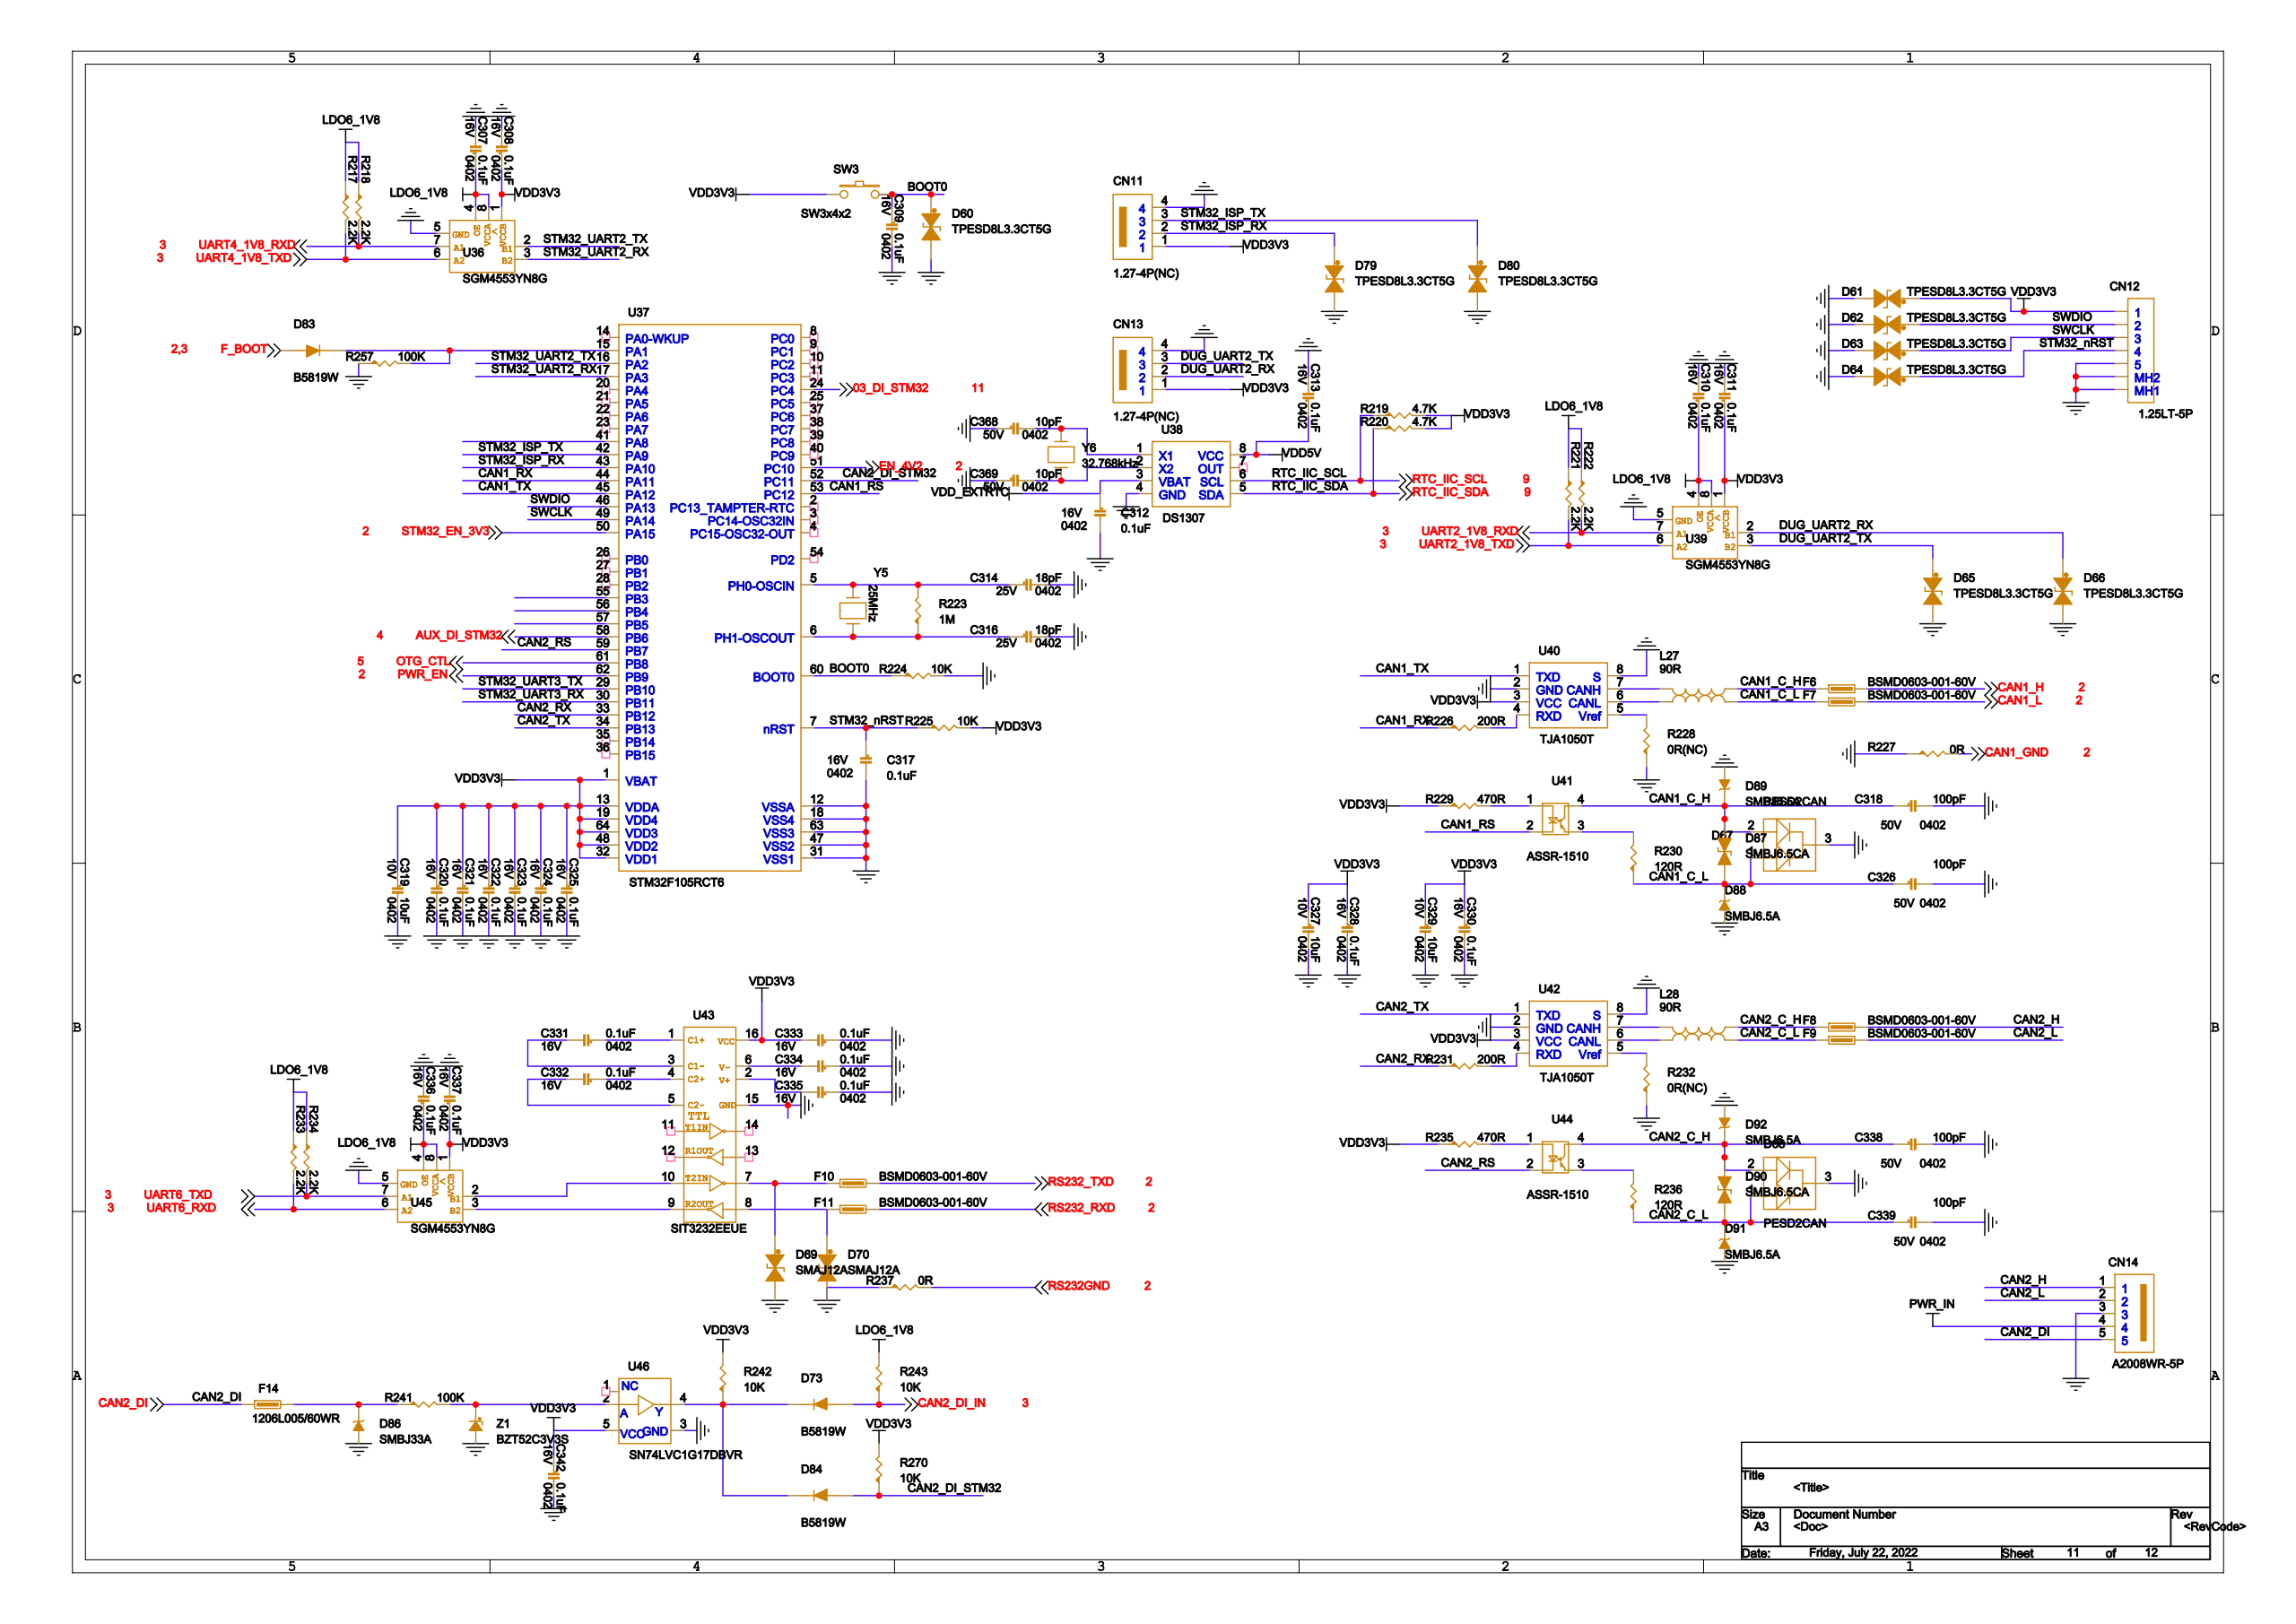Circuit board | Cadence Allegro | 970 parts | 627 nets | one sheet of the schematic
Parts on this sheet (reference | value | footprint):
C307 | 0.1uF | C0402
C308 | 0.1uF | C0402
C309 | 0.1uF | C0402
C310 | 0.1uF | C0402
C311 | 0.1uF | C0402
C312 | 0.1uF | C0402
C313 | 0.1uF | C0402
C314 | 18pF | C0402
C316 | 18pF | C0402
C317 | 0.1uF | C0402
C318 | 100pF | C0402
C319 | 10uF | C0402
C320 | 0.1uF | C0402
C321 | 0.1uF | C0402
C322 | 0.1uF | C0402
C323 | 0.1uF | C0402
C324 | 0.1uF | C0402
C325 | 0.1uF | C0402
C326 | 100pF | C0402
C327 | 10uF | C0402
C328 | 0.1uF | C0402
C329 | 10uF | C0402
C330 | 0.1uF | C0402
C331 | 0.1uF | C0402
C332 | 0.1uF | C0402
C333 | 0.1uF | C0402
C334 | 0.1uF | C0402
C335 | 0.1uF | C0402
C336 | 0.1uF | C0402
C337 | 0.1uF | C0402
C338 | 100pF | C0402
C339 | 100pF | C0402
C342 | 0.1uF | C0402
C368 | 10pF | C0402
C369 | 10pF | C0402
CN11 | 1.27-4P(NC) | SIP4_1P27
CN12 | 1.25LT-5P | PH125_5P_SMD_B
CN13 | 1.27-4P(NC) | SIP4_1P27
CN14 | A2008WR-5P | A2008WR_5P
D60 | TPESD8L3.3CT5G | DFN1006_2L
D61 | TPESD8L3.3CT5G | DFN1006_2L
D62 | TPESD8L3.3CT5G | DFN1006_2L
D63 | TPESD8L3.3CT5G | DFN1006_2L
D64 | TPESD8L3.3CT5G | DFN1006_2L
D65 | TPESD8L3.3CT5G | DFN1006_2L
D66 | TPESD8L3.3CT5G | DFN1006_2L
D67 | PESD2CAN | SOT-23
D68 | PESD2CAN | SOT-23
D69 | SMAJ12A | SMA
D70 | SMAJ12A | SMA
D73 | B5819W | SOD-123
D79 | TPESD8L3.3CT5G | DFN1006_2L
D80 | TPESD8L3.3CT5G | DFN1006_2L
D83 | B5819W | SOD-123
D84 | B5819W | SOD-123
D86 | SMBJ33A | SMB
D87 | SMBJ6.5CA | SMB
D88 | SMBJ6.5A | SMB
D89 | SMBJ6.5A | SMB
D90 | SMBJ6.5CA | SMB
D91 | SMBJ6.5A | SMB
D92 | SMBJ6.5A | SMB
F6 | BSMD0603-001-60V | R0603
F7 | BSMD0603-001-60V | R0603
F8 | BSMD0603-001-60V | R0603
F9 | BSMD0603-001-60V | R0603
F10 | BSMD0603-001-60V | R0603
F11 | BSMD0603-001-60V | R0603
F14 | 1206L005/60WR | R1206
L27 | 90R | WCM2012
L28 | 90R | WCM2012
R217 | 2.2K | R0402
R218 | 2.2K | R0402
R219 | 4.7K | R0402
R220 | 4.7K | R0402
R221 | 2.2K | R0402
R222 | 2.2K | R0402
R223 | 1M | R0402
R224 | 10K | R0402
R225 | 10K | R0402
R226 | 200R | R0402
R227 | 0R | R0402
R228 | 0R(NC) | R0402
R229 | 470R | R0402
R230 | 120R | R0603
R231 | 200R | R0402
R232 | 0R(NC) | R0402
R233 | 2.2K | R0402
R234 | 2.2K | R0402
R235 | 470R | R0402
R236 | 120R | R0603
R237 | 0R | R0402
R241 | 100K | R0402
R242 | 10K | R0402
R243 | 10K | R0402
R257 | 100K | R0402
R270 | 10K | R0402
SW3 | SW3x4x2 | SW3X4X2
U36 | SGM4553YN8G | SOT23_8
U37 | STM32F105RCT6 | LQFP64_12X12_0P5
U38 | DS1307 | SO8
U39 | SGM4553YN8G | SOT23_8
U40 | TJA1050T | SO8
U41 | ASSR-1510 | SO4
U42 | TJA1050T | SO8
U43 | SIT3232EEUE | TSSOP16_6P5MM
U44 | ASSR-1510 | SO4
U45 | SGM4553YN8G | SOT23_8
U46 | SN74LVC1G17DBVR | SOT23-5
Y5 | 25MHz | X3225
Y6 | 32.768kHz | X3215
Z1 | BZT52C3V3S | SOD323
Nets of these parts (net: part-pin ...):
VDD5V: C313-1 U38-8
VDD3V3: C308-1 C311-1 C319-1 C320-1 C321-1 C322-1 C323-1 C324-1 C325-1 C327-1 C328-1 C329-1 C330-1 C333-2 C337-1 C342-1 CN11-1 CN12-1 CN13-1 D61-2 R219-2 R220-2 R225-2 R229-1 R235-1 R242-2 R270-2 SW3-1 U36-1 U39-1 U40-3 U42-3 U43-16 U45-1 U46-5 U37-1 U37-13 U37-19 U37-32 U37-48 U37-64
GND: C307-2 C308-2 C309-2 C310-2 C311-2 C312-2 C313-2 C314-2 C316-2 C317-2 C318-2 C319-2 C320-2 C321-2 C322-2 C323-2 C324-2 C325-2 C326-2 C327-2 C328-2 C329-2 C330-2 C333-1 C334-1 C335-1 C336-2 C337-2 C338-2 C339-2 C342-2 C368-1 C369-1 CN11-4 CN12-5 CN12-MH1 CN12-MH2 CN13-4 CN14-3 D60-1 D61-1 D62-1 D63-1 D64-1 D65-1 D66-1 D67-3 D68-3 D69-1 D70-1 D79-1 D80-1 D86-1 D88-1 D89-1 D91-1 D92-1 R224-2 R227-1 R228-1 R232-1 R237-1 R257-1 U36-5 U38-4 U39-5 U40-2 U40-8 U42-2 U42-8 U43-15 U45-5 U46-3 Y5-2 Y5-4 Z1-1 U37-12 U37-18 U37-31 U37-47 U37-63
LDO6_1V8: C307-1 C310-1 C336-1 R217-1 R218-1 R221-1 R222-1 R233-1 R234-1 R243-2 U36-4 U36-8 U39-4 U39-8 U45-4 U45-8
CAN2_H: CN14-1 F8-2
CAN2_L: CN14-2 F9-2
PWR_IN: CN14-4
CAN2_DI: CN14-5 F14-1
N19340957: D86-2 F14-2 R241-1
CAN1_C_L: C326-1 D67-1 D87-1 D88-2 F7-1 L27-4 R230-1
CAN1_C_H: C318-1 D67-2 D87-2 D89-2 F6-1 L27-2 U41-4
CAN2_C_L: C339-1 D68-1 D90-1 D91-2 F9-1 L28-4 R236-1
CAN2_C_H: C338-1 D68-2 D90-2 D92-2 F8-1 L28-2 U44-4
RTC_IIC_SDA: R220-1 U38-5
RTC_IIC_SCL: R219-1 U38-6
OTG_CTL: U37-61
N19340755: R241-2 U46-2 Z1-2
N19340673: D73-2 D84-2 R242-1 U46-4
N19538177: C368-2 U38-1 Y6-2
VDD_EXTRTC: C312-1 U38-3
N19538168: C369-2 U38-2 Y6-1
RS232GND: R237-2
RS232_TXD: F10-2
RS232_RXD: F11-2
CAN1_H: F6-2
CAN1_L: F7-2
CAN1_GND: R227-2
N19319390: C316-1 R223-1 Y5-1 U37-6
N19319387: C314-1 R223-2 Y5-3 U37-5
SWDIO: CN12-2 D62-2 U37-46
SWCLK: CN12-3 D63-2 U37-49
STM32_NRST: C317-1 CN12-4 D64-2 R225-1 U37-7
DUG_UART2_RX: CN13-2 D66-2 U39-2
DUG_UART2_TX: CN13-3 D65-2 U39-3
STM32_ISP_RX: CN11-2 D79-2 U37-43
STM32_ISP_TX: CN11-3 D80-2 U37-42
BOOT0: C309-1 D60-2 R224-1 SW3-2 U37-60
03_DI_STM32: U37-24
CAN2_DI_STM32: D84-1 R270-1 U37-52
AUX_DI_STM32: U37-58
F_BOOT: D83-1
N19476671: D83-2 R257-2 U37-15
PWR_EN: U37-62
CAN2_DI_IN: D73-1 R243-1
N19337291: D69-2 F10-1 U43-7
N19337298: D70-2 F11-1 U43-8
N19323301: L27-1 U40-7
N19323304: L27-3 U40-6
N19324266: L28-1 U42-7
N19324268: L28-3 U42-6
EN_4V2: U37-51
CAN1_RX: R226-1 U37-44
N19322436: R226-2 U40-4
CAN2_RX: R231-1 U37-33
N19324224: R231-2 U42-4
UART6_RXD: R233-2 U45-6
UART4_1V8_TXD: R217-2 U36-6
UART4_1V8_RXD: R218-2 U36-7
UART2_1V8_TXD: R221-2 U39-6
UART2_1V8_RXD: R222-2 U39-7
UART6_TXD: R234-2 U45-7
N19322586: R228-2 U40-5
N19324248: R232-2 U42-5
N19323409: R229-2 U41-1
N19324337: R235-2 U44-1
N19323390: R230-2 U41-3
N19324316: R236-2 U44-3
STM32_UART2_TX: U36-2 U37-16
STM32_UART2_RX: U36-3 U37-17
N19337098: U43-10 U45-2
N19337109: U43-9 U45-3
CAN1_TX: U40-1 U37-45
STM32_EN_3V3: U37-50
STM32_UART3_TX: U37-29
STM32_UART3_RX: U37-30
CAN2_TX: U42-1 U37-34
CAN2_RS: U44-2 U37-59
CAN1_RS: U41-2 U37-53
N19337373: C331-1 U43-1
N19337376: C331-2 U43-3
N19337411: C332-1 U43-4
N19337402: C332-2 U43-5
N19337451: C335-2 U43-2
N19337431: C334-2 U43-6